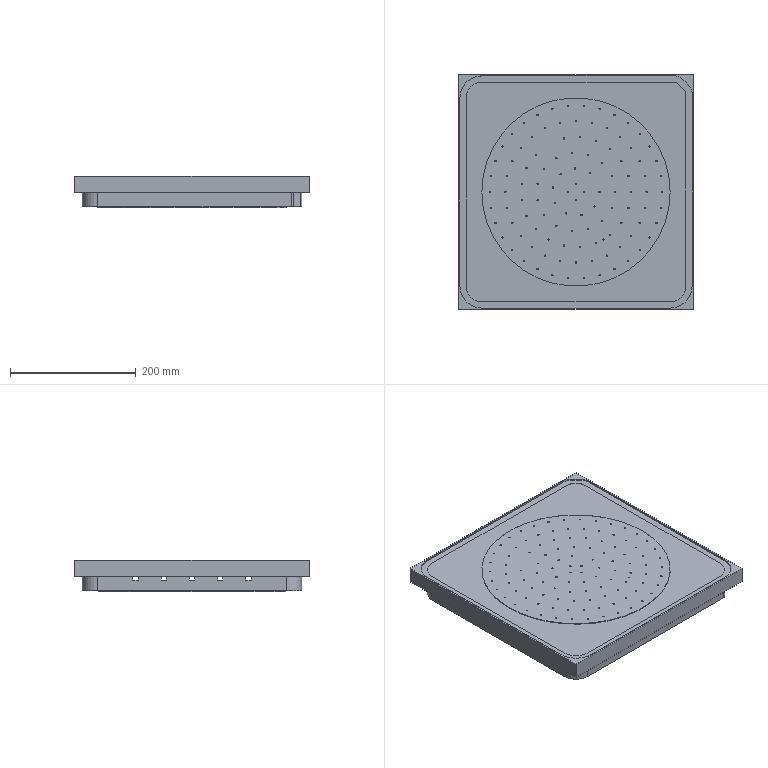NC program | NX | posted with a generic post | part box 374 x 374 x 49.5 mm
Lines 2422 to 3349 of 17720:
(CAVITY_MILL_1 , TOOL : D8)
N4824 M6
N4826 G53
N4828 G17 G0 G90 X125.288 Y90.15 S7000 M3 M8
N4830 G43 Z80. H0
N4832 Z1.
N4834 G94 G1 X105.342 Z-0.045 F4500.
N4836 X104.182 Y90.473 Z-0.108
N4838 X103.17 Y91.125 Z-0.171
N4840 X102.844 Y91.491 Z-0.197
N4842 X101.982 Y92.46 Z-0.265
N4844 X101.1 Y93.414 Z-0.333
N4846 X101.099 Y93.415
N4848 X98.455 Y90.972
N4850 X98.452 Y90.976
N4852 X98.448 Y90.97
N4854 X97.57 Y91.666
N4856 G2 X94.435 Y90.15 R4.
N4858 G1 X70.35
N4860 Y89.03
N4862 X74.962
N4864 G3 X73.863 Y86.138 R5.12
N4866 G1 X74.981 Y86.075
N4868 G2 X78.975 Y89.85 R4.
N4870 G1 X102.039
N4872 G2 X105.1 Y88.425 R4.
N4874 X107.569 Y85.404 R137.35
N4876 X127.68 Y50.624 R137.35
N4878 X123.962 Y45.15 R4.
N4880 G1 X105.79
N4882 G2 X104.495 Y45.365 R4.
N4884 G1 X104.132 Y44.306
N4886 G3 X105.272 Y44.056 R5.12
N4888 X104.809 Y43.374 R5.12
N4890 G1 X105.783 Y42.822
N4892 G2 X109.263 Y44.85 R4.
N4894 G1 X126.939
N4896 G2 X130.747 Y42.075 R4.
N4898 X137.283 Y4.274 R137.35
N4900 X133.285 Y0.15 R4.
N4902 G1 X116.576
N4904 G2 X113.332 Y1.81 R4.
N4906 G1 X112.423 Y1.155
N4908 G3 X113.578 Y0. R5.12
N4910 X112.423 Y-1.155 R5.12
N4912 G1 X113.332 Y-1.81
N4914 G2 X116.576 Y-0.15 R4.
N4916 G1 X133.285
N4918 G2 X137.283 Y-4.274 R4.
N4920 X130.747 Y-42.075 R137.35
N4922 X126.939 Y-44.85 R4.
N4924 G1 X109.263
N4926 G2 X105.783 Y-42.822 R4.
N4928 G1 X104.809 Y-43.374
N4930 G3 X105.272 Y-44.056 R5.12
N4932 X104.132 Y-44.306 R5.12
N4934 G1 X104.495 Y-45.365
N4936 G2 X105.79 Y-45.15 R4.
N4938 G1 X123.962
N4940 G2 X127.68 Y-50.624 R4.
N4942 X105.1 Y-88.425 R137.35
N4944 X102.039 Y-89.85 R4.
N4946 G1 X78.975
N4948 G2 X74.981 Y-86.075 R4.
N4950 G1 X73.863 Y-86.138
N4952 G3 X74.962 Y-89.03 R5.12
N4954 G1 X70.35
N4956 Y-90.15
N4958 X94.435
N4960 G2 X97.268 Y-96.974 R4.
N4962 X-97.268 Y-96.974 R137.35
N4964 X-94.435 Y-90.15 R4.
N4966 G1 X-73.863
N4968 Y-86.138
N4970 G3 X-70.35 Y-89.03 R113.47
N4972 G1 X-69.655 Y-88.151
N4974 G2 X-100.126 Y-50.964 R112.35
N4976 X-99.939 Y-47.008 R4.
N4978 G1 X-102.012 Y-45.694
N4980 G3 X-100.57 Y-45.965 R5.12
N4982 G1 X-100.523 Y-44.846
N4984 G2 X-103.834 Y-42.822 R4.
N4986 G1 X-104.809 Y-43.374
N4988 G3 X-104.132 Y-44.306 R5.12
N4990 X-105.272 Y-44.056 R5.12
N4992 G1 X-105.385 Y-45.171
N4994 G2 X-102.162 Y-47.465 R4.
N4996 G3 X-76.267 Y-82.906 R112.65
N4998 G2 X-78.975 Y-89.85 R4.
N5000 G1 X-102.039
N5002 G2 X-105.1 Y-88.425 R4.
N5004 X-127.68 Y-50.624 R137.35
N5006 X-123.962 Y-45.15 R4.
N5008 G1 X-105.79
N5010 G2 X-105.385 Y-45.171 R4.
N5012 G1 X-105.272 Y-44.056
N5014 G3 X-104.809 Y-43.374 R5.12
N5016 G1 X-105.783 Y-42.822
N5018 G2 X-109.263 Y-44.85 R4.
N5020 G1 X-126.939
N5022 G2 X-130.747 Y-42.075 R4.
N5024 X-137.283 Y-4.274 R137.35
N5026 X-133.285 Y-0.15 R4.
N5028 G1 X-116.576
N5030 G2 X-114.111 Y-1. R4.
N5032 G1 X-112.423 Y1.155
N5034 G3 X-111.269 Y0. R5.12
N5036 G1 X-110.613 Y0.908
N5038 G2 X-112.268 Y4.303 R4.
N5040 X-104.059 Y42.358 R112.35
N5042 X-103.705 Y43.035 R4.
N5044 G1 X-105.272 Y44.056
N5046 G3 X-104.132 Y44.306 R5.12
N5048 G1 X-104.495 Y45.365
N5050 G2 X-105.79 Y45.15 R4.
N5052 G1 X-123.962
N5054 G2 X-127.68 Y50.624 R4.
N5056 X-105.1 Y88.425 R137.35
N5058 X-102.039 Y89.85 R4.
N5060 G1 X-78.975
N5062 G2 X-75.84 Y88.334 R4.
N5064 G1 X-74.962 Y89.03
N5066 X-70.35
N5068 G3 X-73.863 Y86.138 R113.47
N5070 G1 X-73.134 Y85.288
N5072 G2 X-68.543 Y89.019 R112.35
N5074 X-66.102 Y89.85 R4.
N5076 G1 X-64.524
N5078 Y90.97
N5080 G2 X-58.698 Y94.834 R111.53
N5082 G3 X-57.636 Y90.97 R5.12
N5084 G1 X-56.759 Y91.666
N5086 G2 X-55.603 Y97.626 R4.
N5088 X55.603 Y97.626 R112.35
N5090 X57.588 Y94.684 R4.
N5092 G1 X58.698 Y94.834
N5094 G2 X64.524 Y90.97 R111.53
N5096 G1 X57.636
N5098 Y89.85
N5100 X66.102
N5102 G2 X68.512 Y89.042 R4.
N5104 G1 X68.543 Y89.019
N5106 G2 X100.126 Y50.964 R112.35
N5108 X100.166 Y47.417 R4.
N5110 G1 X101.175 Y46.932
N5112 G3 X102.012 Y45.694 R5.12
N5114 X100.57 Y45.965 R5.12
N5116 G1 X100.523 Y44.846
N5118 G2 X104.059 Y42.358 R4.
N5120 X104.25 Y41.887 R112.35
N5122 X112.268 Y4.303 R112.35
N5124 X108.27 Y0.15 R4.
N5126 G1 X91.556
N5128 G2 X88.31 Y1.812 R4.
N5130 G1 X87.401 Y1.158
N5132 G3 X88.557 Y0. R5.12
N5134 X87.401 Y-1.158 R5.12
N5136 G1 X88.31 Y-1.812
N5138 G2 X91.556 Y-0.15 R4.
N5140 G1 X108.27
N5142 G2 X112.268 Y-4.303 R4.
N5144 X104.25 Y-41.887 R112.35
N5146 X104.059 Y-42.358 R112.35
N5148 X100.523 Y-44.846 R4.
N5150 G1 X100.57 Y-45.965
N5152 G3 X102.012 Y-45.694 R5.12
N5154 X101.175 Y-46.932 R5.12
N5156 X100.57 Y-45.965 R5.12
N5158 G1 X99.693 Y-46.662
N5160 G2 X100.16 Y-50.896 R4.
N5162 G1 X100.126 Y-50.964
N5164 G2 X68.543 Y-89.019 R112.35
N5166 G1 X68.512 Y-89.042
N5168 G2 X66.102 Y-89.85 R4.
N5170 G1 X57.636
N5172 Y-90.97
N5174 X64.524
N5176 G2 X58.698 Y-94.834 R111.53
N5178 G3 X57.636 Y-90.97 R5.12
N5180 G1 X56.759 Y-91.666
N5182 G2 X55.603 Y-97.626 R4.
N5184 X-55.603 Y-97.626 R112.35
N5186 X-57.464 Y-93.03 R4.
N5188 G1 X-64.524 Y-90.97
N5190 X-57.636
N5192 G3 X-58.698 Y-94.834 R5.12
N5194 G2 X-64.524 Y-90.97 R111.53
N5196 G1 X-57.464 Y-93.03
N5198 G2 X-53.624 Y-90.15 R4.
N5200 G1 X-27.25
N5202 Y-84.169
N5204 G3 X27.25 Y-84.169 R88.47
N5206 G1 X26.905 Y-83.103
N5208 G2 X-70.547 Y-51.509 R87.35
N5210 X-70.847 Y-47.27 R4.
N5212 G1 X-73.386 Y-45.917
N5214 G3 X-72.653 Y-45.97 R5.12
N5216 G1 X-71.329
N5218 Y-44.85
N5220 X-72.653
N5222 G2 X-76.14 Y-42.81 R4.
N5224 G1 X-77.116 Y-43.359
N5226 G3 X-76.624 Y-44.083 R5.12
N5228 X-77.356 Y-44.03 R5.12
N5230 G1 X-78.03
N5232 G3 X-77.361 Y-42.922 R5.12
N5234 X-77.116 Y-43.359 R88.47
N5236 G1 X-76.14 Y-42.81
N5238 G2 X-87.242 Y-4.349 R87.35
N5240 X-85.712 Y-1. R4.
N5242 G1 X-87.401 Y1.158
N5244 G3 X-86.245 Y0. R5.12
N5246 G1 X-85.589 Y0.908
N5248 G2 X-87.242 Y4.349 R4.
N5250 X-76.14 Y42.81 R87.35
N5252 G1 X-76.096 Y42.886
N5254 X-78.03 Y44.03
N5256 X-77.356
N5258 G3 X-76.624 Y44.083 R5.12
N5260 X-77.116 Y43.359 R5.12
N5262 X-77.361 Y42.922 R88.47
N5264 X-78.03 Y44.03 R5.12
N5266 G1 X-76.096 Y42.886
N5268 G2 X-72.653 Y44.85 R4.
N5270 G1 X-72.217
N5272 Y47.667
N5274 G3 X-71.329 Y45.97 R5.12
N5276 G1 X-70.451 Y46.666
N5278 G2 X-71.314 Y49.008 R4.
N5280 X-70.547 Y51.509 R4.
N5282 X26.268 Y83.307 R87.35
N5284 G1 X28.073 Y89.03
N5286 X28.027 Y88.971
N5288 G3 X27.25 Y84.169 R5.12
N5290 X-27.25 Y84.169 R88.47
N5292 X-28.073 Y89.03 R5.12
N5294 G1 X28.073
N5296 X26.268 Y83.307
N5298 G2 X70.547 Y51.509 R87.35
N5300 X70.922 Y47.419 R4.
N5302 G1 X73.035 Y46.404
N5304 G3 X73.386 Y45.917 R5.12
N5306 X72.653 Y45.97 R5.12
N5308 G1 X71.329
N5310 Y44.85
N5312 X72.653
N5314 G2 X75.755 Y43.376 R4.
N5316 G1 X76.624 Y44.083
N5318 G3 X77.356 Y44.03 R5.12
N5320 G1 X78.03
N5322 G3 X77.361 Y42.922 R5.12
N5324 X77.116 Y43.359 R88.47
N5326 X76.624 Y44.083 R5.12
N5328 G1 X75.755 Y43.376
N5330 G2 X76.14 Y42.81 R4.
N5332 X76.946 Y41.343 R87.35
N5334 X87.242 Y4.349 R87.35
N5336 X83.247 Y0.15 R4.
N5338 G1 X66.521
N5340 G2 X63.271 Y1.817 R4.
N5342 G1 X62.361 Y1.164
N5344 G3 X63.522 Y0. R5.12
N5346 X62.361 Y-1.164 R5.12
N5348 G1 X63.271 Y-1.817
N5350 G2 X66.521 Y-0.15 R4.
N5352 G1 X83.247
N5354 G2 X87.242 Y-4.349 R4.
N5356 X76.946 Y-41.343 R87.35
N5358 X76.381 Y-42.378 R87.35
N5360 G1 X77.361 Y-42.922
N5362 G3 X78.03 Y-44.03 R5.12
N5364 G1 X77.356
N5366 G3 X76.624 Y-44.083 R5.12
N5368 X77.116 Y-43.359 R5.12
N5370 X77.361 Y-42.922 R88.47
N5372 G1 X76.381 Y-42.378
N5374 G2 X76.14 Y-42.81 R87.35
N5376 X72.653 Y-44.85 R4.
N5378 G1 X71.329
N5380 Y-45.97
N5382 X72.653
N5384 G3 X73.386 Y-45.917 R5.12
N5386 X73.035 Y-46.404 R5.12
N5388 G2 X72.217 Y-47.667 R86.53
N5390 G3 X71.329 Y-45.97 R5.12
N5392 G1 Y-44.85
N5394 X52.664
N5396 G2 X48.752 Y-41.686 R4.
N5398 G1 X47.657 Y-41.92
N5400 G3 X48.651 Y-44.03 R5.12
N5402 G1 X45.714
N5404 G3 X47.657 Y-41.92 R63.47
N5406 G1 X46.816 Y-41.18
N5408 G2 X44.522 Y-43.65 R62.35
N5410 X41.665 Y-44.85 R4.
N5412 G1 X35.461
N5414 Y-45.97
N5416 X40.899
N5418 G2 X36.557 Y-49.493 R61.53
N5420 G3 X35.461 Y-45.97 R5.12
N5422 G1 X34.583 Y-46.666
N5424 G2 X33.604 Y-52.519 R4.
N5426 X-33.604 Y-52.519 R62.35
N5428 X-35.239 Y-47.874 R4.
N5430 G1 X-40.899 Y-45.97
N5432 X-35.461
N5434 Y-44.85
N5436 X-41.665
N5438 G2 X-43.931 Y-44.146 R4.
N5440 X-44.522 Y-43.65 R4.
N5442 X-46.816 Y-41.18 R62.35
N5444 G1 X-47.657 Y-41.92
N5446 G3 X-45.714 Y-44.03 R63.47
N5448 G1 X-48.651
N5450 G3 X-47.657 Y-41.92 R5.12
N5452 G1 X-46.816 Y-41.18
N5454 G2 X-47.573 Y-40.303 R62.35
N5456 X-62.192 Y-4.434 R62.35
N5458 X-60.668 Y-1. R4.
N5460 G1 X-62.361 Y1.164
N5462 G3 X-61.201 Y0. R5.12
N5464 G1 X-60.545 Y0.908
N5466 G2 X-62.192 Y4.434 R4.
N5468 X-46.229 Y41.838 R62.35
N5470 G1 X-48.651 Y44.03
N5472 X-45.714
N5474 G3 X-47.657 Y41.92 R63.47
N5476 X-48.651 Y44.03 R5.12
N5478 G1 X-46.229 Y41.838
N5480 G2 X-44.522 Y43.65 R62.35
N5482 X-41.665 Y44.85 R4.
N5484 G1 X-36.557
N5486 Y49.493
N5488 G3 X-35.461 Y45.97 R5.12
N5490 G1 X-34.583 Y46.666
N5492 G2 X-33.604 Y52.519 R4.
N5494 X33.604 Y52.519 R62.35
N5496 X34.583 Y46.666 R4.
N5498 G1 X35.461 Y45.97
N5500 G3 X36.557 Y49.493 R5.12
N5502 G2 X40.899 Y45.97 R61.53
N5504 G1 X35.461
N5506 Y44.85
N5508 X41.665
N5510 G2 X44.522 Y43.65 R4.
N5512 X44.908 Y43.253 R62.35
N5514 G1 X45.714 Y44.03
N5516 X48.651
N5518 G3 X47.657 Y41.92 R5.12
N5520 X45.714 Y44.03 R63.47
N5522 G1 X44.908 Y43.253
N5524 G2 X62.192 Y4.434 R62.35
N5526 X58.202 Y0.15 R4.
N5528 G1 X41.443
N5530 G2 X38.18 Y1.836 R4.
N5532 G1 X37.267 Y1.188
N5534 G3 X38.444 Y0. R5.12
N5536 X37.267 Y-1.188 R5.12
N5538 X36.089 Y0. R5.12
N5540 G1 X35.433 Y-0.908
N5542 G2 X37.06 Y-4.648 R4.
N5544 X-3.581 Y-37.178 R37.35
N5546 G1 X-3.688 Y-38.293
N5548 G3 X3.688 Y-38.293 R38.47
N5550 X4.111 Y-44.03 R5.12
N5552 G1 X-4.111
N5554 G3 X-3.688 Y-38.293 R5.12
N5556 G1 X-3.581 Y-37.178
N5558 G2 X-37.06 Y-4.648 R37.35
N5560 X-35.556 Y-1. R4.
N5562 G1 X-37.267 Y1.188
N5564 G3 X-36.089 Y0. R5.12
N5566 G1 X-35.433 Y0.908
N5568 G2 X-37.06 Y4.648 R4.
N5570 X-3.472 Y37.188 R37.35
N5572 G1 X-4.111 Y44.03
N5574 X4.111
N5576 X4.056 Y43.959
N5578 G3 X3.688 Y38.293 R5.12
N5580 X-3.688 Y38.293 R38.47
N5582 X-4.111 Y44.03 R5.12
N5584 G1 X-3.472 Y37.188
N5586 G2 X37.06 Y4.648 R37.35
N5588 X33.091 Y0.15 R4.
N5590 G1 X16.125
N5592 G2 X12.856 Y1.844 R4.
N5594 G1 X10.244 Y0.
N5596 G3 X11.685 Y1.599 R5.12
N5598 G1 X10.714 Y2.157
N5600 G2 X7.246 Y0.15 R4.
N5602 G1 X-7.246
N5604 G2 X-10.714 Y2.157 R4.
N5606 G1 X-11.685 Y1.599
N5608 G3 X-10.244 Y0. R5.12
N5610 X-11.685 Y-1.599 R5.12
N5612 G1 X-10.714 Y-2.157
N5614 G2 X-7.246 Y-0.15 R4.
N5616 G1 X7.246
N5618 G2 X10.717 Y-6.138 R4.
N5620 X-10.717 Y-6.138 R12.35
N5622 X-10.714 Y-2.157 R4.
N5624 G1 X-11.685 Y-1.599
N5626 G3 X-13.126 Y0. R5.12
N5628 X-11.685 Y1.599 R5.12
N5630 G1 X-10.714 Y2.157
N5632 G2 X-10.717 Y6.138 R4.
N5634 X10.717 Y6.138 R12.35
N5636 X10.714 Y2.157 R4.
N5638 G1 X11.685 Y1.599
N5640 G3 X13.126 Y0. R5.12
N5642 X11.685 Y-1.599 R5.12
N5644 X10.244 Y0. R5.12
N5646 G1 X12.856 Y1.844
N5648 G2 X12.251 Y3.153 R4.
N5650 G3 X-12.251 Y3.153 R12.65
N5652 G2 X-16.125 Y0.15 R4.
N5654 G1 X-33.091
N5656 G2 X-35.433 Y0.908 R4.
N5658 G1 X-36.089 Y0.
N5660 G3 X-37.267 Y-1.188 R5.12
N5662 X-38.444 Y0. R5.12
N5664 X-37.267 Y1.188 R5.12
N5666 G1 X-35.556 Y-1.
N5668 G2 X-33.091 Y-0.15 R4.
N5670 G1 X-16.125
N5672 G2 X-12.251 Y-3.153 R4.
N5674 G3 X12.251 Y-3.153 R12.65
N5676 G2 X16.125 Y-0.15 R4.
N5678 G1 X33.091
N5680 G2 X35.433 Y-0.908 R4.
N5682 G1 X36.089 Y0.
N5684 G3 X37.267 Y1.188 R5.12
N5686 G1 X38.18 Y1.836
N5688 G2 X37.463 Y3.751 R4.
N5690 G3 X7.344 Y36.927 R37.65
N5692 G2 X8.124 Y44.85 R4.
N5694 G1 X35.461
N5696 Y45.97
N5698 X34.583 Y46.666
N5700 G2 X31.448 Y45.15 R4.
N5702 G1 X-31.448
N5704 G2 X-34.583 Y46.666 R4.
N5706 G1 X-35.461 Y45.97
N5708 X-40.899
N5710 G2 X-36.557 Y49.493 R61.53
N5712 G1 Y44.85
N5714 X-8.124
N5716 G2 X-7.344 Y36.927 R4.
N5718 G3 X-37.463 Y3.751 R37.65
N5720 G2 X-41.443 Y0.15 R4.
N5722 G1 X-58.202
N5724 G2 X-60.545 Y0.908 R4.
N5726 G1 X-61.201 Y0.
N5728 G3 X-62.361 Y-1.164 R5.12
N5730 X-63.522 Y0. R5.12
N5732 X-62.361 Y1.164 R5.12
N5734 G1 X-60.668 Y-1.
N5736 G2 X-58.202 Y-0.15 R4.
N5738 G1 X-41.443
N5740 G2 X-37.463 Y-3.751 R4.
N5742 G3 X-7.344 Y-36.927 R37.65
N5744 G2 X-8.124 Y-44.85 R4.
N5746 G1 X-35.461
N5748 Y-45.97
N5750 G3 X-36.557 Y-49.493 R5.12
N5752 G2 X-40.899 Y-45.97 R61.53
N5754 G1 X-35.239 Y-47.874
N5756 G2 X-31.448 Y-45.15 R4.
N5758 G1 X31.448
N5760 G2 X34.583 Y-46.666 R4.
N5762 G1 X35.461 Y-45.97
N5764 Y-44.85
N5766 X8.124
N5768 G2 X7.344 Y-36.927 R4.
N5770 G3 X37.463 Y-3.751 R37.65
N5772 G2 X41.443 Y-0.15 R4.
N5774 G1 X58.202
N5776 G2 X62.192 Y-4.434 R4.
N5778 X46.816 Y-41.18 R62.35
N5780 G1 X47.657 Y-41.92
N5782 X48.752 Y-41.686
N5784 G2 X48.665 Y-40.745 R4.
N5786 X49.503 Y-38.398 R4.
N5788 G3 X62.528 Y-3.901 R62.65
N5790 G2 X63.271 Y-1.817 R4.
N5792 G1 X62.361 Y-1.164
N5794 G3 X61.201 Y0. R5.12
N5796 X62.361 Y1.164 R5.12
N5798 G1 X63.271 Y1.817
N5800 G2 X62.528 Y3.901 R4.
N5802 G3 X49.503 Y38.398 R62.65
N5804 G2 X52.664 Y44.85 R4.
N5806 G1 X71.329
N5808 Y45.97
N5810 G3 X72.217 Y47.667 R5.12
N5812 G2 X73.035 Y46.404 R86.53
N5814 G1 X70.922 Y47.419
N5816 G2 X67.316 Y45.15 R4.
N5818 G1 X45.017
N5820 G2 X42.315 Y46.2 R4.
N5822 G3 X-42.315 Y46.2 R62.65
N5824 G2 X-45.017 Y45.15 R4.
N5826 G1 X-67.316
N5828 G2 X-70.451 Y46.666 R4.
N5830 G1 X-71.329 Y45.97
N5832 X-72.653
N5834 G3 X-73.386 Y45.917 R5.12
N5836 X-73.035 Y46.404 R5.12
N5838 G2 X-72.217 Y47.667 R86.53
N5840 G1 Y44.85
N5842 X-52.664
N5844 G2 X-49.503 Y38.398 R4.
N5846 G3 X-62.528 Y3.901 R62.65
N5848 G2 X-66.521 Y0.15 R4.
N5850 G1 X-83.247
N5852 G2 X-85.589 Y0.908 R4.
N5854 G1 X-86.245 Y0.
N5856 G3 X-87.401 Y-1.158 R5.12
N5858 X-88.557 Y0. R5.12
N5860 X-87.401 Y1.158 R5.12
N5862 G1 X-85.712 Y-1.
N5864 G2 X-83.247 Y-0.15 R4.
N5866 G1 X-66.521
N5868 G2 X-62.528 Y-3.901 R4.
N5870 G3 X-49.503 Y-38.398 R62.65
N5872 G2 X-52.664 Y-44.85 R4.
N5874 G1 X-71.329
N5876 Y-45.97
N5878 G3 X-72.217 Y-47.667 R5.12
N5880 G2 X-73.035 Y-46.404 R86.53
N5882 G3 X-73.386 Y-45.917 R5.12
N5884 G1 X-70.847 Y-47.27
N5886 G2 X-67.316 Y-45.15 R4.
N5888 G1 X-45.017
N5890 G2 X-42.315 Y-46.2 R4.
N5892 G3 X42.315 Y-46.2 R62.65
N5894 G2 X45.017 Y-45.15 R4.
N5896 G1 X67.316
N5898 G2 X70.547 Y-51.509 R4.
N5900 X26.905 Y-83.103 R87.35
N5902 G1 X27.25 Y-84.169
N5904 G3 X28.073 Y-89.03 R5.12
N5906 G1 X-28.073
N5908 G3 X-27.25 Y-84.169 R5.12
N5910 G1 Y-90.15
N5912 X53.624
N5914 G2 X56.759 Y-91.666 R4.
N5916 G1 X57.636 Y-90.97
N5918 Y-89.85
N5920 X32.086
N5922 G2 X30.685 Y-82.103 R4.
N5924 G3 X73.98 Y-47.005 R87.65
N5926 G2 X77.356 Y-45.15 R4.
N5928 G1 X96.561
N5930 G2 X99.693 Y-46.662 R4.
N5932 G1 X100.57 Y-45.965
N5934 X100.523 Y-44.846
N5936 X100.354 Y-44.85
N5938 X82.043
N5940 G2 X78.434 Y-39.124 R4.
N5942 G1 X78.462 Y-39.067
N5944 G3 X87.56 Y-3.969 R87.65
N5946 G2 X88.31 Y-1.812 R4.
N5948 G1 X87.401 Y-1.158
N5950 G3 X86.245 Y0. R5.12
N5952 X87.401 Y1.158 R5.12
N5954 G1 X88.31 Y1.812
N5956 G2 X87.56 Y3.969 R4.
N5958 G3 X78.462 Y39.067 R87.65
N5960 G2 X82.033 Y44.85 R4.
N5962 G1 X82.043
N5964 X100.354
N5966 X100.523 Y44.846
N5968 X100.57 Y45.965
N5970 G3 X101.175 Y46.932 R5.12
N5972 G1 X100.166 Y47.417
N5974 G2 X96.561 Y45.15 R4.
N5976 G1 X77.356
N5978 G2 X73.98 Y47.005 R4.
N5980 G3 X30.685 Y82.103 R87.65
N5982 G2 X32.086 Y89.85 R4.
N5984 G1 X57.636
N5986 Y90.97
N5988 G3 X58.698 Y94.834 R5.12
N5990 G1 X57.588 Y94.684
N5992 G2 X53.624 Y90.15 R4.
N5994 G1 X-53.624
N5996 G2 X-56.759 Y91.666 R4.
N5998 G1 X-57.636 Y90.97
N6000 X-64.524
N6002 Y89.85
N6004 X-32.086
N6006 G2 X-30.685 Y82.103 R4.
N6008 G3 X-73.98 Y47.005 R87.65
N6010 G2 X-77.356 Y45.15 R4.
N6012 G1 X-96.561
N6014 G2 X-100.166 Y47.417 R4.
N6016 G1 X-101.175 Y46.932
N6018 G3 X-100.57 Y45.965 R5.12
N6020 X-102.012 Y45.694 R5.12
N6022 X-101.175 Y46.932 R5.12
N6024 G1 X-100.166 Y47.417
N6026 G2 X-100.16 Y50.896 R4.
N6028 G1 X-100.126 Y50.964
N6030 G2 X-73.134 Y85.288 R112.35
N6032 G1 X-73.863 Y86.138
N6034 G3 X-74.962 Y89.03 R5.12
N6036 G1 X-75.84 Y88.334
N6038 G2 X-76.267 Y82.906 R4.
N6040 G3 X-102.162 Y47.465 R112.65
N6042 G2 X-104.495 Y45.365 R4.
N6044 G1 X-104.132 Y44.306
N6046 G3 X-104.809 Y43.374 R5.12
N6048 X-105.272 Y44.056 R5.12
N6050 G1 X-106.145 Y43.355
N6052 G2 X-105.517 Y39.449 R4.
N6054 G3 X-112.579 Y4.008 R112.65
N6056 G2 X-116.576 Y0.15 R4.
N6058 G1 X-133.285
N6060 G2 X-137.283 Y4.274 R4.
N6062 X-130.747 Y42.075 R137.35
N6064 X-126.939 Y44.85 R4.
N6066 G1 X-109.263
N6068 G2 X-106.145 Y43.355 R4.
N6070 G1 X-105.272 Y44.056
N6072 X-103.705 Y43.035
N6074 G2 X-100.354 Y44.85 R4.
N6076 G1 X-82.043
N6078 G2 X-78.462 Y39.067 R4.
N6080 G3 X-87.56 Y3.969 R87.65
N6082 G2 X-91.556 Y0.15 R4.
N6084 G1 X-108.27
N6086 G2 X-110.613 Y0.908 R4.
N6088 G1 X-111.269 Y0.
N6090 G3 X-112.423 Y-1.155 R5.12
N6092 X-113.578 Y0. R5.12
N6094 X-112.423 Y1.155 R5.12
N6096 G1 X-114.111 Y-1.
N6098 G2 X-112.579 Y-4.008 R4.
N6100 G3 X-105.517 Y-39.449 R112.65
N6102 G2 X-105.783 Y-42.822 R4.
N6104 G1 X-104.809 Y-43.374
N6106 X-103.834 Y-42.822
N6108 G2 X-104.059 Y-42.358 R4.
N6110 X-112.268 Y-4.303 R112.35
N6112 X-108.27 Y-0.15 R4.
N6114 G1 X-91.556
N6116 G2 X-87.56 Y-3.969 R4.
N6118 G3 X-78.462 Y-39.067 R87.65
N6120 G2 X-82.033 Y-44.85 R4.
N6122 G1 X-82.043
N6124 X-100.354
N6126 X-100.523 Y-44.846
N6128 X-100.57 Y-45.965
N6130 G3 X-101.175 Y-46.932 R5.12
N6132 X-102.012 Y-45.694 R5.12
N6134 G1 X-99.939 Y-47.008
N6136 G2 X-96.561 Y-45.15 R4.
N6138 G1 X-77.356
N6140 G2 X-73.98 Y-47.005 R4.
N6142 G3 X-30.685 Y-82.103 R87.65
N6144 G2 X-32.086 Y-89.85 R4.
N6146 G1 X-66.102
N6148 G2 X-68.543 Y-89.019 R4.
N6150 X-69.655 Y-88.151 R112.35
N6152 G1 X-70.35 Y-89.03
N6154 X-74.962
N6156 G3 X-73.863 Y-86.138 R5.12
N6158 G1 Y-90.15
N6160 X-68.869
N6162 G2 X-66.508 Y-90.922 R4.
N6164 G3 X66.508 Y-90.922 R112.65
N6166 G2 X68.869 Y-90.15 R4.
N6168 G1 X70.35
N6170 Y-89.03
N6172 G3 X73.863 Y-86.138 R113.47
N6174 G1 X74.981 Y-86.075
N6176 G2 X76.267 Y-82.906 R4.
N6178 G3 X102.162 Y-47.465 R112.65
N6180 G2 X104.495 Y-45.365 R4.
N6182 G1 X104.132 Y-44.306
N6184 G3 X104.809 Y-43.374 R5.12
N6186 G1 X105.783 Y-42.822
N6188 G2 X105.517 Y-39.449 R4.
N6190 G3 X112.579 Y-4.008 R112.65
N6192 G2 X113.332 Y-1.81 R4.
N6194 G1 X112.423 Y-1.155
N6196 G3 X111.269 Y0. R5.12
N6198 X112.423 Y1.155 R5.12
N6200 G1 X113.332 Y1.81
N6202 G2 X112.579 Y4.008 R4.
N6204 G3 X105.517 Y39.449 R112.65
N6206 G2 X105.783 Y42.822 R4.
N6208 G1 X104.809 Y43.374
N6210 G3 X104.132 Y44.306 R5.12
N6212 G1 X104.495 Y45.365
N6214 G2 X102.162 Y47.465 R4.
N6216 G3 X76.267 Y82.906 R112.65
N6218 G2 X74.981 Y86.075 R4.
N6220 G1 X73.863 Y86.138
N6222 G3 X70.35 Y89.03 R113.47
N6224 G1 Y90.15
N6226 X68.869
N6228 G2 X66.508 Y90.922 R4.
N6230 G1 X66.459 Y90.958
N6232 G3 X-66.508 Y90.922 R112.65
N6234 G2 X-68.869 Y90.15 R4.
N6236 G1 X-94.435
N6238 G2 X-97.268 Y96.974 R4.
N6240 X97.268 Y96.974 R137.35
N6242 X97.57 Y91.666 R4.
N6244 G1 X98.448 Y90.97
N6246 X98.457
N6248 X98.455 Y90.972
N6250 X101.099 Y93.415
N6252 G3 X-101.096 Y93.419 R137.65
N6254 G1 X-98.452 Y90.976
N6256 X-98.457 Y90.97
N6258 X-98.448
N6260 X-98.452 Y90.976
N6262 X-101.096 Y93.419
N6264 G3 X-102.844 Y91.491 R137.65
N6266 G2 X-105.832 Y90.15 R4.
N6268 G1 X-175.
N6270 G2 X-178.696 Y92.62 R4.
N6272 G1 Y90.607
N6274 G3 X-177.999 Y90. R5.12
N6276 X-178.696 Y89.393 R5.12
N6278 G1 Y87.38
N6280 G2 X-175. Y89.85 R4.
N6282 G1 X-112.67
N6284 G2 X-109.488 Y83.426 R4.
N6286 G3 X-129.098 Y47.762 R137.65
N6288 G2 X-132.85 Y45.15 R4.
N6290 G1 X-175.
N6292 G2 X-178.696 Y47.62 R4.
N6294 G1 Y45.606
N6296 G3 X-177.999 Y45. R5.12
N6298 X-178.696 Y44.394 R5.12
N6300 G1 Y42.381
N6302 G2 X-175. Y44.85 R4.
N6304 G1 X-135.632
N6306 G2 X-131.802 Y39.696 R4.
N6308 G3 X-137.591 Y4.033 R137.65
N6310 G2 X-141.589 Y0.15 R4.
N6312 G1 X-175.
N6314 G2 X-178.695 Y2.619 R4.
N6316 G1 Y0.606
N6318 G3 X-177.999 Y0. R5.12
N6320 X-178.695 Y-0.606 R5.12
N6322 G1 Y-2.619
N6324 G2 X-175. Y-0.15 R4.
N6326 G1 X-141.589
N6328 G2 X-137.591 Y-4.033 R4.
N6330 G3 X-131.802 Y-39.696 R137.65
N6332 G2 X-131.875 Y-42.224 R4.
N6334 X-133.205 Y-44.03 R4.
N6336 X-135.632 Y-44.85 R4.
N6338 G1 X-175.
N6340 G2 X-178.695 Y-42.382 R4.
N6342 G1 Y-44.394
N6344 G3 X-177.999 Y-45. R5.12
N6346 X-178.695 Y-45.606 R5.12
N6348 G1 Y-47.618
N6350 G2 X-175. Y-45.15 R4.
N6352 G1 X-132.85
N6354 G2 X-129.098 Y-47.762 R4.
N6356 G3 X-109.488 Y-83.426 R137.65
N6358 G2 X-112.67 Y-89.85 R4.
N6360 G1 X-175.
N6362 G2 X-178.695 Y-87.382 R4.
N6364 G1 Y-89.394
N6366 G3 X-177.999 Y-90. R5.12
N6368 X-178.695 Y-90.606 R5.12
N6370 G1 Y-92.618
N6372 G2 X-175. Y-90.15 R4.
N6374 G1 X-105.832
N6376 G2 X-102.844 Y-91.491 R4.
N6378 G3 X-101.102 Y-93.413 R137.65
N6380 G1 X-98.457 Y-90.97
N6382 X-98.452 Y-90.976
N6384 X-98.448 Y-90.97
N6386 X-98.457
N6388 X-101.102 Y-93.413
N6390 G3 X101.096 Y-93.419 R137.65
N6392 G1 X98.452 Y-90.976
N6394 X98.457 Y-90.97
N6396 X98.448
N6398 X98.452 Y-90.976
N6400 X101.096 Y-93.419
N6402 G3 X102.844 Y-91.491 R137.65
N6404 G2 X105.832 Y-90.15 R4.
N6406 G1 X175.
N6408 G2 X178.696 Y-92.62 R4.
N6410 G1 Y-90.607
N6412 G3 X177.999 Y-90. R5.12
N6414 X178.696 Y-89.393 R5.12
N6416 G1 Y-87.38
N6418 G2 X175. Y-89.85 R4.
N6420 G1 X112.67
N6422 G2 X109.488 Y-83.426 R4.
N6424 G3 X129.098 Y-47.762 R137.65
N6426 G2 X132.85 Y-45.15 R4.
N6428 G1 X175.
N6430 G2 X178.696 Y-47.62 R4.
N6432 G1 Y-45.606
N6434 G3 X177.999 Y-45. R5.12
N6436 X178.696 Y-44.394 R5.12
N6438 G1 Y-42.381
N6440 G2 X175. Y-44.85 R4.
N6442 G1 X135.632
N6444 G2 X133.205 Y-44.03 R4.
N6446 X131.802 Y-39.696 R4.
N6448 G3 X137.591 Y-4.033 R137.65
N6450 G2 X141.589 Y-0.15 R4.
N6452 G1 X175.
N6454 G2 X178.695 Y-2.619 R4.
N6456 G1 Y-0.606
N6458 G3 X177.999 Y0. R5.12
N6460 X178.695 Y0.606 R5.12
N6462 G1 Y2.619
N6464 G2 X175. Y0.15 R4.
N6466 G1 X141.589
N6468 G2 X137.591 Y4.033 R4.
N6470 G3 X131.802 Y39.696 R137.65
N6472 G2 X135.632 Y44.85 R4.
N6474 G1 X175.
N6476 G2 X178.695 Y42.382 R4.
N6478 G1 Y44.394
N6480 G3 X177.999 Y45. R5.12
N6482 X178.695 Y45.606 R5.12
N6484 G1 Y47.618
N6486 G2 X175. Y45.15 R4.
N6488 G1 X132.85
N6490 G2 X129.098 Y47.762 R4.
N6492 G3 X109.488 Y83.426 R137.65
N6494 G2 X112.67 Y89.85 R4.
N6496 G1 X175.
N6498 G2 X178.695 Y87.382 R4.
N6500 G1 Y89.394
N6502 G3 X177.999 Y90. R5.12
N6504 X178.695 Y90.606 R5.12
N6506 G1 Y92.618
N6508 G2 X175. Y90.15 R4.
N6510 G1 X105.832
N6512 G2 X102.844 Y91.491 R4.
N6514 G3 X101.099 Y93.415 R137.65
N6516 X100.543 Y93.672 R0.8
N6518 G1 Z0.667
N6520 G0 Z3.
N6522 X125.288 Y90.15
N6524 Z0.667
N6526 G1 X105.832 Z-0.353
N6528 X105.342 Z-0.379
N6530 X104.182 Y90.473 Z-0.442
N6532 X103.17 Y91.125 Z-0.505
N6534 X101.982 Y92.46 Z-0.599
N6536 X101.1 Y93.414 Z-0.667
N6538 X101.099 Y93.415
N6540 X98.455 Y90.972
N6542 X98.452 Y90.976
N6544 X98.448 Y90.97
N6546 X97.57 Y91.666
N6548 G2 X94.435 Y90.15 R4.
N6550 G1 X74.962
N6552 Y89.03
N6554 G3 X73.863 Y86.138 R5.12
N6556 G1 X74.981 Y86.075
N6558 G2 X78.975 Y89.85 R4.
N6560 G1 X102.039
N6562 G2 X105.1 Y88.425 R4.
N6564 X107.569 Y85.404 R137.35
N6566 X127.68 Y50.624 R137.35
N6568 X123.962 Y45.15 R4.
N6570 G1 X105.79
N6572 G2 X104.495 Y45.365 R4.
N6574 G1 X104.132 Y44.306
N6576 G3 X105.272 Y44.056 R5.12
N6578 X104.809 Y43.374 R5.12
N6580 G1 X105.783 Y42.822
N6582 G2 X109.263 Y44.85 R4.
N6584 G1 X126.939
N6586 G2 X130.747 Y42.075 R4.
N6588 X137.283 Y4.274 R137.35
N6590 X133.285 Y0.15 R4.
N6592 G1 X116.576
N6594 G2 X113.332 Y1.81 R4.
N6596 G1 X112.423 Y1.155
N6598 G3 X113.578 Y0. R5.12
N6600 X112.423 Y-1.155 R5.12
N6602 G1 X113.332 Y-1.81
N6604 G2 X116.576 Y-0.15 R4.
N6606 G1 X133.285
N6608 G2 X137.283 Y-4.274 R4.
N6610 X130.747 Y-42.075 R137.35
N6612 X126.939 Y-44.85 R4.
N6614 G1 X109.263
N6616 G2 X105.783 Y-42.822 R4.
N6618 G1 X104.809 Y-43.374
N6620 G3 X105.272 Y-44.056 R5.12
N6622 X104.132 Y-44.306 R5.12
N6624 G1 X104.495 Y-45.365
N6626 G2 X105.79 Y-45.15 R4.
N6628 G1 X123.962
N6630 G2 X127.68 Y-50.624 R4.
N6632 X105.1 Y-88.425 R137.35
N6634 X102.039 Y-89.85 R4.
N6636 G1 X78.975
N6638 G2 X74.981 Y-86.075 R4.
N6640 G1 X73.863 Y-86.138
N6642 G3 X74.962 Y-89.03 R5.12
N6644 G1 X70.35
N6646 Y-90.15
N6648 X94.435
N6650 G2 X97.268 Y-96.974 R4.
N6652 X-97.268 Y-96.974 R137.35
N6654 X-94.435 Y-90.15 R4.
N6656 G1 X-73.863
N6658 Y-86.138
N6660 G3 X-70.35 Y-89.03 R113.47
N6662 G1 X-69.655 Y-88.151
N6664 G2 X-100.126 Y-50.964 R112.35
N6666 X-99.939 Y-47.008 R4.
N6668 G1 X-102.012 Y-45.694
N6670 G3 X-100.57 Y-45.965 R5.12
N6672 G1 X-100.523 Y-44.846